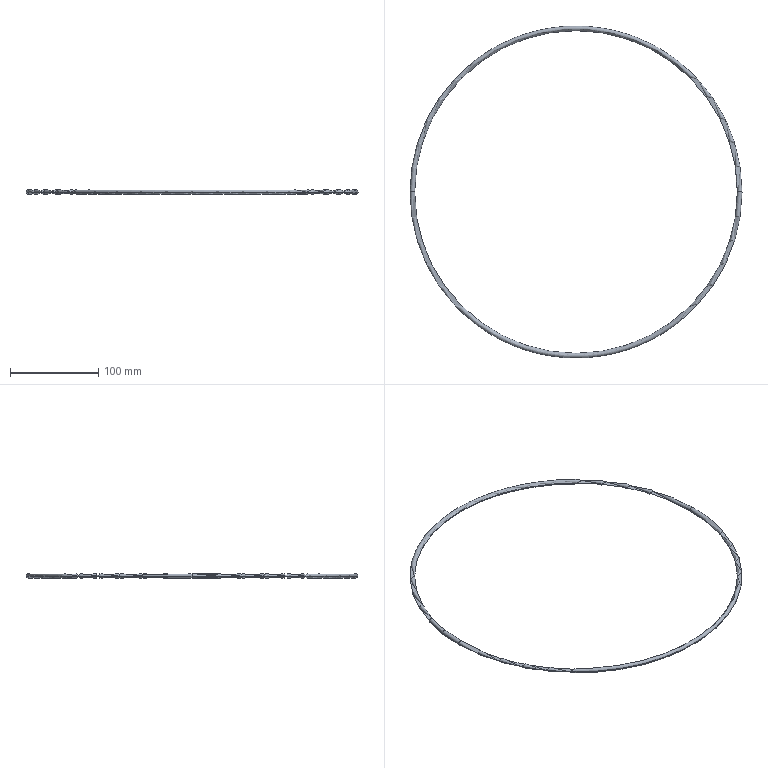Part | SolidWorks | features RefAxis 1, Sweep 1 | 1 solid | 4 faces | box 375.6 x 375.6 x 5.3 mm | volume 25665 mm3 | torus 4
STEP:
#1=CARTESIAN_POINT('',(187.8,0.,0.));
#2=VERTEX_POINT('',#1);
#3=CARTESIAN_POINT('',(182.5,0.,0.));
#4=VERTEX_POINT('',#3);
#5=CARTESIAN_POINT('',(185.15,0.,0.));
#6=DIRECTION('',(0.,1.,0.));
#7=DIRECTION('',(-1.,0.,0.));
#8=AXIS2_PLACEMENT_3D('',#5,#6,#7);
#9=CIRCLE('',#8,2.65);
#10=EDGE_CURVE('',#2,#4,#9,.T.);
#11=ORIENTED_EDGE('',*,*,#10,.F.);
#12=CARTESIAN_POINT('',(-187.8,0.,0.));
#13=VERTEX_POINT('',#12);
#14=CARTESIAN_POINT('',(0.,0.,0.));
#15=DIRECTION('',(0.,0.,-1.));
#16=DIRECTION('',(-1.,0.,0.));
#17=AXIS2_PLACEMENT_3D('',#14,#15,#16);
#18=CIRCLE('',#17,187.8);
#19=EDGE_CURVE('',#2,#13,#18,.T.);
#20=ORIENTED_EDGE('',*,*,#19,.T.);
#21=CARTESIAN_POINT('',(-182.5,0.,0.));
#22=VERTEX_POINT('',#21);
#23=CARTESIAN_POINT('',(-185.15,0.,0.));
#24=DIRECTION('',(0.,-1.,0.));
#25=DIRECTION('',(0.,0.,-1.));
#26=AXIS2_PLACEMENT_3D('',#23,#24,#25);
#27=CIRCLE('',#26,2.65);
#28=EDGE_CURVE('',#13,#22,#27,.T.);
#29=ORIENTED_EDGE('',*,*,#28,.T.);
#30=CARTESIAN_POINT('',(0.,0.,0.));
#31=DIRECTION('',(0.,0.,-1.));
#32=DIRECTION('',(-1.,0.,0.));
#33=AXIS2_PLACEMENT_3D('',#30,#31,#32);
#34=CIRCLE('',#33,182.5);
#35=EDGE_CURVE('',#4,#22,#34,.T.);
#36=ORIENTED_EDGE('',*,*,#35,.F.);
#37=EDGE_LOOP('',(#11,#20,#29,#36));
#38=FACE_OUTER_BOUND('',#37,.T.);
#39=CARTESIAN_POINT('',(0.,0.,0.));
#40=DIRECTION('',(0.,0.,-1.));
#41=DIRECTION('',(-1.,0.,0.));
#42=AXIS2_PLACEMENT_3D('',#39,#40,#41);
#43=TOROIDAL_SURFACE('',#42,185.15,2.65);
#44=ADVANCED_FACE('',(#38),#43,.T.);
#45=ORIENTED_EDGE('',*,*,#28,.F.);
#46=CARTESIAN_POINT('',(0.,0.,0.));
#47=DIRECTION('',(0.,0.,-1.));
#48=DIRECTION('',(-1.,0.,0.));
#49=AXIS2_PLACEMENT_3D('',#46,#47,#48);
#50=CIRCLE('',#49,187.8);
#51=EDGE_CURVE('',#13,#2,#50,.T.);
#52=ORIENTED_EDGE('',*,*,#51,.T.);
#53=ORIENTED_EDGE('',*,*,#10,.T.);
#54=CARTESIAN_POINT('',(0.,0.,0.));
#55=DIRECTION('',(0.,0.,-1.));
#56=DIRECTION('',(-1.,0.,0.));
#57=AXIS2_PLACEMENT_3D('',#54,#55,#56);
#58=CIRCLE('',#57,182.5);
#59=EDGE_CURVE('',#22,#4,#58,.T.);
#60=ORIENTED_EDGE('',*,*,#59,.F.);
#61=EDGE_LOOP('',(#45,#52,#53,#60));
#62=FACE_OUTER_BOUND('',#61,.T.);
#63=CARTESIAN_POINT('',(0.,0.,0.));
#64=DIRECTION('',(0.,0.,-1.));
#65=DIRECTION('',(-1.,0.,0.));
#66=AXIS2_PLACEMENT_3D('',#63,#64,#65);
#67=TOROIDAL_SURFACE('',#66,185.15,2.65);
#68=ADVANCED_FACE('',(#62),#67,.T.);
#69=ORIENTED_EDGE('',*,*,#51,.F.);
#70=CARTESIAN_POINT('',(-185.15,0.,0.));
#71=DIRECTION('',(0.,-1.,0.));
#72=DIRECTION('',(0.,0.,-1.));
#73=AXIS2_PLACEMENT_3D('',#70,#71,#72);
#74=CIRCLE('',#73,2.65);
#75=EDGE_CURVE('',#22,#13,#74,.T.);
#76=ORIENTED_EDGE('',*,*,#75,.F.);
#77=ORIENTED_EDGE('',*,*,#59,.T.);
#78=CARTESIAN_POINT('',(185.15,0.,0.));
#79=DIRECTION('',(0.,1.,0.));
#80=DIRECTION('',(-1.,0.,0.));
#81=AXIS2_PLACEMENT_3D('',#78,#79,#80);
#82=CIRCLE('',#81,2.65);
#83=EDGE_CURVE('',#4,#2,#82,.T.);
#84=ORIENTED_EDGE('',*,*,#83,.T.);
#85=EDGE_LOOP('',(#69,#76,#77,#84));
#86=FACE_OUTER_BOUND('',#85,.T.);
#87=CARTESIAN_POINT('',(0.,0.,0.));
#88=DIRECTION('',(0.,0.,-1.));
#89=DIRECTION('',(-1.,0.,0.));
#90=AXIS2_PLACEMENT_3D('',#87,#88,#89);
#91=TOROIDAL_SURFACE('',#90,185.15,2.65);
#92=ADVANCED_FACE('',(#86),#91,.T.);
#93=ORIENTED_EDGE('',*,*,#19,.F.);
#94=ORIENTED_EDGE('',*,*,#83,.F.);
#95=ORIENTED_EDGE('',*,*,#35,.T.);
#96=ORIENTED_EDGE('',*,*,#75,.T.);
#97=EDGE_LOOP('',(#93,#94,#95,#96));
#98=FACE_OUTER_BOUND('',#97,.T.);
#99=CARTESIAN_POINT('',(0.,0.,0.));
#100=DIRECTION('',(0.,0.,-1.));
#101=DIRECTION('',(-1.,0.,0.));
#102=AXIS2_PLACEMENT_3D('',#99,#100,#101);
#103=TOROIDAL_SURFACE('',#102,185.15,2.65);
#104=ADVANCED_FACE('',(#98),#103,.T.);
#105=CLOSED_SHELL('',(#44,#68,#92,#104));
#106=MANIFOLD_SOLID_BREP('',#105);
#107=CARTESIAN_POINT('',(0.,0.,0.));
#108=DIRECTION('',(0.,0.,1.));
#109=DIRECTION('',(1.,0.,0.));
#110=AXIS2_PLACEMENT_3D('',#107,#108,#109);
#111=(LENGTH_UNIT()NAMED_UNIT(*)SI_UNIT(.MILLI.,.METRE.));
#112=UNCERTAINTY_MEASURE_WITH_UNIT(LENGTH_MEASURE(0.00001),#111,'','');
#113=(NAMED_UNIT(*)PLANE_ANGLE_UNIT()SI_UNIT($,.RADIAN.));
#114=(NAMED_UNIT(*)SI_UNIT($,.STERADIAN.)SOLID_ANGLE_UNIT());
#115=(GEOMETRIC_REPRESENTATION_CONTEXT(3)GLOBAL_UNCERTAINTY_ASSIGNED_CONTEXT((#112))GLOBAL_UNIT_ASSIGNED_CONTEXT((#111,#113,#114))REPRESENTATION_CONTEXT('',''));
#116=ADVANCED_BREP_SHAPE_REPRESENTATION('',(#106,#110),#115);